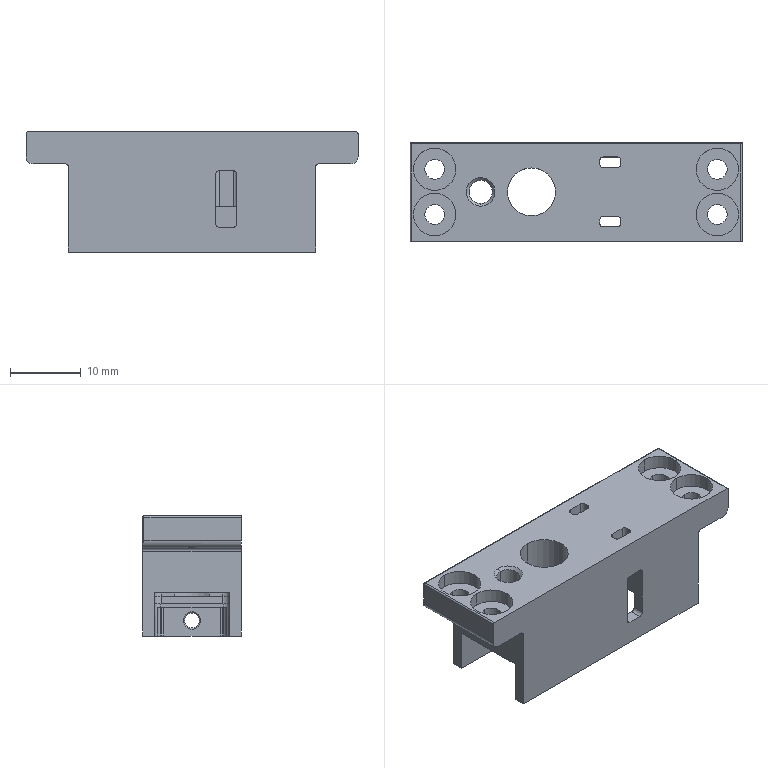NC program | NX | posted with a generic post | part box 47 x 14 x 17 mm
Lines 6223 to 7148 of 12912:
(CAVITY_MILL_COPY_COPY_COPY , TOOL : D1)
N12390 T22 M6
N12392 G54
N12394 G17 G0 G90 X9.057 Y-4.65 B0. C0. S9200 M3
N12396 G43 Z30. H22
N12398 Z0.936
N12400 G94 G1 Z-0.064 F1000.
N12402 G3 X9.492 Y-4.75 R1.
N12404 G1 X9.9 F850.
N12406 G3 X10.141 Y-4.628 R0.3
N12408 G2 X10.544 Y-4.425 R0.5
N12410 G1 X10.7
N12412 G3 X10.981 Y-4.231 R0.3
N12414 G2 X11.293 Y-3.885 R0.64
N12416 G3 X11.732 Y-3.456 R1.
N12418 G1 Z0.936
N12420 G0 Z30.
N12422 X9.057 Y-4.65
N12424 Z0.872
N12426 G1 Z-0.128 F1000.
N12428 G3 X9.492 Y-4.75 R1.
N12430 G1 X9.9 F850.
N12432 G3 X10.141 Y-4.628 R0.3
N12434 G2 X10.544 Y-4.425 R0.5
N12436 G1 X10.7
N12438 G3 X10.981 Y-4.231 R0.3
N12440 G2 X11.293 Y-3.885 R0.64
N12442 G3 X11.732 Y-3.456 R1.
N12444 G1 Z0.872
N12446 G0 Z30.
N12448 X9.057 Y-4.65
N12450 Z0.808
N12452 G1 Z-0.192 F1000.
N12454 G3 X9.492 Y-4.75 R1.
N12456 G1 X9.9 F850.
N12458 G3 X10.141 Y-4.628 R0.3
N12460 G2 X10.544 Y-4.425 R0.5
N12462 G1 X10.7
N12464 G3 X10.981 Y-4.231 R0.3
N12466 G2 X11.293 Y-3.885 R0.64
N12468 G3 X11.732 Y-3.456 R1.
N12470 G1 Z0.808
N12472 G0 Z30.
N12474 X9.057 Y-4.65
N12476 Z0.744
N12478 G1 Z-0.256 F1000.
N12480 G3 X9.492 Y-4.75 R1.
N12482 G1 X9.9 F850.
N12484 G3 X10.141 Y-4.628 R0.3
N12486 G2 X10.544 Y-4.425 R0.5
N12488 G1 X10.7
N12490 G3 X10.981 Y-4.231 R0.3
N12492 G2 X11.293 Y-3.885 R0.64
N12494 G3 X11.732 Y-3.456 R1.
N12496 G1 Z0.744
N12498 G0 Z30.
N12500 X9.057 Y-4.65
N12502 Z0.68
N12504 G1 Z-0.32 F1000.
N12506 G3 X9.492 Y-4.75 R1.
N12508 G1 X9.9 F850.
N12510 G3 X10.141 Y-4.628 R0.3
N12512 G2 X10.544 Y-4.425 R0.5
N12514 G1 X10.7
N12516 G3 X10.981 Y-4.231 R0.3
N12518 G2 X11.293 Y-3.885 R0.64
N12520 G3 X11.732 Y-3.456 R1.
N12522 G1 Z0.68
N12524 G0 Z30.
N12526 X9.057 Y-4.65
N12528 Z0.616
N12530 G1 Z-0.384 F1000.
N12532 G3 X9.492 Y-4.75 R1.
N12534 G1 X9.9 F850.
N12536 G3 X10.141 Y-4.628 R0.3
N12538 G2 X10.544 Y-4.425 R0.5
N12540 G1 X10.7
N12542 G3 X10.981 Y-4.231 R0.3
N12544 G2 X11.293 Y-3.885 R0.64
N12546 G3 X11.732 Y-3.456 R1.
N12548 G1 Z0.616
N12550 G0 Z30.
N12552 X9.057 Y-4.65
N12554 Z0.552
N12556 G1 Z-0.448 F1000.
N12558 G3 X9.492 Y-4.75 R1.
N12560 G1 X9.9 F850.
N12562 G3 X10.141 Y-4.628 R0.3
N12564 G2 X10.544 Y-4.425 R0.5
N12566 G1 X10.7
N12568 G3 X10.981 Y-4.231 R0.3
N12570 G2 X11.293 Y-3.885 R0.64
N12572 G3 X11.732 Y-3.456 R1.
N12574 G1 Z0.552
N12576 G0 Z30.
N12578 X9.057 Y-4.65
N12580 Z0.488
N12582 G1 Z-0.513 F1000.
N12584 G3 X9.492 Y-4.75 R1.
N12586 G1 X9.9 F850.
N12588 G3 X10.141 Y-4.628 R0.3
N12590 G2 X10.544 Y-4.425 R0.5
N12592 G1 X10.7
N12594 G3 X10.981 Y-4.231 R0.3
N12596 G2 X11.293 Y-3.885 R0.64
N12598 G3 X11.732 Y-3.456 R1.
N12600 G1 Z0.488
N12602 G0 Z30.
N12604 X9.057 Y-4.65
N12606 Z0.423
N12608 G1 Z-0.577 F1000.
N12610 G3 X9.492 Y-4.75 R1.
N12612 G1 X9.9 F850.
N12614 G3 X10.141 Y-4.628 R0.3
N12616 G2 X10.544 Y-4.425 R0.5
N12618 G1 X10.7
N12620 G3 X10.981 Y-4.231 R0.3
N12622 G2 X11.293 Y-3.885 R0.64
N12624 G3 X11.732 Y-3.456 R1.
N12626 G1 Z0.423
N12628 G0 Z30.
N12630 X9.057 Y-4.65
N12632 Z0.359
N12634 G1 Z-0.641 F1000.
N12636 G3 X9.492 Y-4.75 R1.
N12638 G1 X9.9 F850.
N12640 G3 X10.141 Y-4.628 R0.3
N12642 G2 X10.544 Y-4.425 R0.5
N12644 G1 X10.7
N12646 G3 X10.981 Y-4.231 R0.3
N12648 G2 X11.293 Y-3.885 R0.64
N12650 G3 X11.732 Y-3.456 R1.
N12652 G1 Z0.359
N12654 G0 Z30.
N12656 X9.057 Y-4.65
N12658 Z0.295
N12660 G1 Z-0.705 F1000.
N12662 G3 X9.492 Y-4.75 R1.
N12664 G1 X9.9 F850.
N12666 G3 X10.141 Y-4.628 R0.3
N12668 G2 X10.544 Y-4.425 R0.5
N12670 G1 X10.7
N12672 G3 X10.981 Y-4.231 R0.3
N12674 G2 X11.293 Y-3.885 R0.64
N12676 G3 X11.732 Y-3.456 R1.
N12678 G1 Z0.295
N12680 G0 Z30.
N12682 X9.057 Y-4.65
N12684 Z0.231
N12686 G1 Z-0.769 F1000.
N12688 G3 X9.492 Y-4.75 R1.
N12690 G1 X9.9 F850.
N12692 G3 X10.141 Y-4.628 R0.3
N12694 G2 X10.544 Y-4.425 R0.5
N12696 G1 X10.7
N12698 G3 X10.981 Y-4.231 R0.3
N12700 G2 X11.293 Y-3.885 R0.64
N12702 G3 X11.732 Y-3.456 R1.
N12704 G1 Z0.231
N12706 G0 Z30.
N12708 X9.057 Y-4.65
N12710 Z0.167
N12712 G1 Z-0.833 F1000.
N12714 G3 X9.492 Y-4.75 R1.
N12716 G1 X9.9 F850.
N12718 G3 X10.141 Y-4.628 R0.3
N12720 G2 X10.544 Y-4.425 R0.5
N12722 G1 X10.7
N12724 G3 X10.981 Y-4.231 R0.3
N12726 G2 X11.293 Y-3.885 R0.64
N12728 G3 X11.732 Y-3.456 R1.
N12730 G1 Z0.167
N12732 G0 Z30.
N12734 X9.057 Y-4.65
N12736 Z0.103
N12738 G1 Z-0.897 F1000.
N12740 G3 X9.492 Y-4.75 R1.
N12742 G1 X9.9 F850.
N12744 G3 X10.141 Y-4.628 R0.3
N12746 G2 X10.544 Y-4.425 R0.5
N12748 G1 X10.7
N12750 G3 X10.981 Y-4.231 R0.3
N12752 G2 X11.293 Y-3.885 R0.64
N12754 G3 X11.732 Y-3.456 R1.
N12756 G1 Z0.103
N12758 G0 Z30.
N12760 X9.057 Y-4.65
N12762 Z0.039
N12764 G1 Z-0.961 F1000.
N12766 G3 X9.492 Y-4.75 R1.
N12768 G1 X9.9 F850.
N12770 G3 X10.141 Y-4.628 R0.3
N12772 G2 X10.544 Y-4.425 R0.5
N12774 G1 X10.7
N12776 G3 X10.981 Y-4.231 R0.3
N12778 G2 X11.293 Y-3.885 R0.64
N12780 G3 X11.732 Y-3.456 R1.
N12782 G1 Z0.039
N12784 X9.057 Y-4.65 Z-0.025 F8000.
N12786 Z-1.025 F1000.
N12788 G3 X9.492 Y-4.75 R1.
N12790 G1 X9.9 F850.
N12792 G3 X10.141 Y-4.628 R0.3
N12794 G2 X10.544 Y-4.425 R0.5
N12796 G1 X10.7
N12798 G3 X10.981 Y-4.231 R0.3
N12800 G2 X11.293 Y-3.885 R0.64
N12802 G3 X11.732 Y-3.456 R1.
N12804 G1 Z-0.025
N12806 X9.057 Y-4.65 Z-0.089 F8000.
N12808 Z-1.089 F1000.
N12810 G3 X9.492 Y-4.75 R1.
N12812 G1 X9.9 F850.
N12814 G3 X10.141 Y-4.628 R0.3
N12816 G2 X10.544 Y-4.425 R0.5
N12818 G1 X10.7
N12820 G3 X10.981 Y-4.231 R0.3
N12822 G2 X11.293 Y-3.885 R0.64
N12824 G3 X11.732 Y-3.456 R1.
N12826 G1 Z-0.089
N12828 X9.057 Y-4.65 Z-0.153 F8000.
N12830 Z-1.153 F1000.
N12832 G3 X9.492 Y-4.75 R1.
N12834 G1 X9.9 F850.
N12836 G3 X10.141 Y-4.628 R0.3
N12838 G2 X10.544 Y-4.425 R0.5
N12840 G1 X10.7
N12842 G3 X10.981 Y-4.231 R0.3
N12844 G2 X11.293 Y-3.885 R0.64
N12846 G3 X11.732 Y-3.456 R1.
N12848 G1 Z-0.153
N12850 X9.057 Y-4.65 Z-0.217 F8000.
N12852 Z-1.217 F1000.
N12854 G3 X9.492 Y-4.75 R1.
N12856 G1 X9.9 F850.
N12858 G3 X10.141 Y-4.628 R0.3
N12860 G2 X10.544 Y-4.425 R0.5
N12862 G1 X10.7
N12864 G3 X10.981 Y-4.231 R0.3
N12866 G2 X11.293 Y-3.885 R0.64
N12868 G3 X11.732 Y-3.456 R1.
N12870 G1 Z-0.217
N12872 X9.057 Y-4.65 Z-0.281 F8000.
N12874 Z-1.281 F1000.
N12876 G3 X9.492 Y-4.75 R1.
N12878 G1 X9.9 F850.
N12880 G3 X10.141 Y-4.628 R0.3
N12882 G2 X10.544 Y-4.425 R0.5
N12884 G1 X10.7
N12886 G3 X10.981 Y-4.231 R0.3
N12888 G2 X11.293 Y-3.885 R0.64
N12890 G3 X11.732 Y-3.456 R1.
N12892 G1 Z-0.281
N12894 X9.057 Y-4.65 Z-0.345 F8000.
N12896 Z-1.345 F1000.
N12898 G3 X9.492 Y-4.75 R1.
N12900 G1 X9.9 F850.
N12902 G3 X10.141 Y-4.628 R0.3
N12904 G2 X10.544 Y-4.425 R0.5
N12906 G1 X10.7
N12908 G3 X10.981 Y-4.231 R0.3
N12910 G2 X11.293 Y-3.885 R0.64
N12912 G3 X11.732 Y-3.456 R1.
N12914 G1 Z-0.345
N12916 X9.057 Y-4.65 Z-0.409 F8000.
N12918 Z-1.409 F1000.
N12920 G3 X9.492 Y-4.75 R1.
N12922 G1 X9.9 F850.
N12924 G3 X10.141 Y-4.628 R0.3
N12926 G2 X10.544 Y-4.425 R0.5
N12928 G1 X10.71
N12930 G3 X10.981 Y-4.231 R0.3
N12932 G2 X11.293 Y-3.885 R0.64
N12934 G3 X11.732 Y-3.456 R1.
N12936 G1 Z-0.409
N12938 X9.057 Y-4.65 Z-0.473 F8000.
N12940 Z-1.473 F1000.
N12942 G3 X9.492 Y-4.75 R1.
N12944 G1 X9.9 F850.
N12946 G3 X10.141 Y-4.628 R0.3
N12948 G2 X10.544 Y-4.425 R0.5
N12950 G1 X10.71
N12952 G3 X10.981 Y-4.231 R0.3
N12954 G2 X11.293 Y-3.885 R0.64
N12956 G3 X11.732 Y-3.456 R1.
N12958 G1 Z-0.473
N12960 X9.057 Y-4.65 Z-0.538 F8000.
N12962 Z-1.538 F1000.
N12964 G3 X9.492 Y-4.75 R1.
N12966 G1 X9.9 F850.
N12968 G3 X10.141 Y-4.628 R0.3
N12970 G2 X10.544 Y-4.425 R0.5
N12972 G1 X10.711
N12974 G3 X10.981 Y-4.231 R0.3
N12976 G2 X11.293 Y-3.885 R0.64
N12978 G3 X11.732 Y-3.456 R1.
N12980 G1 Z-0.538
N12982 X9.057 Y-4.65 Z-0.602 F8000.
N12984 Z-1.602 F1000.
N12986 G3 X9.492 Y-4.75 R1.
N12988 G1 X9.9 F850.
N12990 G3 X10.141 Y-4.628 R0.3
N12992 G2 X10.544 Y-4.425 R0.5
N12994 G1 X10.711
N12996 G3 X10.981 Y-4.231 R0.3
N12998 G2 X11.293 Y-3.885 R0.64
N13000 G3 X11.732 Y-3.456 R1.
N13002 G1 Z-0.602
N13004 X9.057 Y-4.65 Z-0.666 F8000.
N13006 Z-1.666 F1000.
N13008 G3 X9.492 Y-4.75 R1.
N13010 G1 X9.9 F850.
N13012 G3 X10.141 Y-4.628 R0.3
N13014 G2 X10.544 Y-4.425 R0.5
N13016 G1 X10.711
N13018 G3 X10.981 Y-4.231 R0.3
N13020 G2 X11.293 Y-3.885 R0.64
N13022 G3 X11.732 Y-3.456 R1.
N13024 G1 Z-0.666
N13026 X9.057 Y-4.65 Z-0.73 F8000.
N13028 Z-1.73 F1000.
N13030 G3 X9.492 Y-4.75 R1.
N13032 G1 X9.9 F850.
N13034 G3 X10.141 Y-4.628 R0.3
N13036 G2 X10.544 Y-4.425 R0.5
N13038 G1 X10.711
N13040 G3 X10.981 Y-4.231 R0.3
N13042 G2 X11.293 Y-3.885 R0.64
N13044 G3 X11.732 Y-3.456 R1.
N13046 G1 Z-0.73
N13048 X9.057 Y-4.65 Z-0.794 F8000.
N13050 Z-1.794 F1000.
N13052 G3 X9.492 Y-4.75 R1.
N13054 G1 X9.9 F850.
N13056 G3 X10.141 Y-4.628 R0.3
N13058 G2 X10.544 Y-4.425 R0.5
N13060 G1 X10.711
N13062 G3 X10.981 Y-4.231 R0.3
N13064 G2 X11.293 Y-3.885 R0.64
N13066 G3 X11.732 Y-3.456 R1.
N13068 G1 Z-0.794
N13070 X9.057 Y-4.65 Z-0.858 F8000.
N13072 Z-1.858 F1000.
N13074 G3 X9.492 Y-4.75 R1.
N13076 G1 X9.9 F850.
N13078 G3 X10.141 Y-4.628 R0.3
N13080 G2 X10.544 Y-4.425 R0.5
N13082 G1 X10.712
N13084 G3 X10.981 Y-4.231 R0.3
N13086 G2 X11.293 Y-3.885 R0.64
N13088 G3 X11.732 Y-3.456 R1.
N13090 G1 Z-0.858
N13092 X9.057 Y-4.65 Z-0.922 F8000.
N13094 Z-1.922 F1000.
N13096 G3 X9.492 Y-4.75 R1.
N13098 G1 X9.9 F850.
N13100 G3 X10.141 Y-4.628 R0.3
N13102 G2 X10.544 Y-4.425 R0.5
N13104 G1 X10.712
N13106 G3 X10.981 Y-4.231 R0.3
N13108 G2 X11.293 Y-3.885 R0.64
N13110 G3 X11.732 Y-3.456 R1.
N13112 G1 Z-0.922
N13114 X9.057 Y-4.65 Z-0.986 F8000.
N13116 Z-1.986 F1000.
N13118 G3 X9.492 Y-4.75 R1.
N13120 G1 X9.9 F850.
N13122 G3 X10.141 Y-4.628 R0.3
N13124 G2 X10.544 Y-4.425 R0.5
N13126 G1 X10.712
N13128 G3 X10.981 Y-4.231 R0.3
N13130 G2 X11.293 Y-3.885 R0.64
N13132 G3 X11.732 Y-3.456 R1.
N13134 G1 Z-0.986
N13136 X9.057 Y-4.65 Z-1.05 F8000.
N13138 Z-2.05 F1000.
N13140 G3 X9.492 Y-4.75 R1.
N13142 G1 X9.9 F850.
N13144 G3 X10.141 Y-4.628 R0.3
N13146 G2 X10.544 Y-4.425 R0.5
N13148 G1 X10.712
N13150 G3 X10.981 Y-4.231 R0.3
N13152 G2 X11.293 Y-3.885 R0.64
N13154 G3 X11.732 Y-3.456 R1.
N13156 G1 Z-1.05
N13158 X9.057 Y-4.65 Z-1.114 F8000.
N13160 Z-2.114 F1000.
N13162 G3 X9.492 Y-4.75 R1.
N13164 G1 X9.9 F850.
N13166 G3 X10.141 Y-4.628 R0.3
N13168 G2 X10.544 Y-4.425 R0.5
N13170 G1 X10.712
N13172 G3 X10.981 Y-4.231 R0.3
N13174 G2 X11.293 Y-3.885 R0.64
N13176 G3 X11.732 Y-3.456 R1.
N13178 G1 Z-1.114
N13180 X9.057 Y-4.65 Z-1.178 F8000.
N13182 Z-2.178 F1000.
N13184 G3 X9.492 Y-4.75 R1.
N13186 G1 X9.9 F850.
N13188 G3 X10.141 Y-4.628 R0.3
N13190 G2 X10.544 Y-4.425 R0.5
N13192 G1 X10.713
N13194 G3 X10.981 Y-4.231 R0.3
N13196 G2 X11.293 Y-3.885 R0.64
N13198 G3 X11.732 Y-3.456 R1.
N13200 G1 Z-1.178
N13202 X9.057 Y-4.65 Z-1.242 F8000.
N13204 Z-2.242 F1000.
N13206 G3 X9.492 Y-4.75 R1.
N13208 G1 X9.9 F850.
N13210 G3 X10.141 Y-4.628 R0.3
N13212 G2 X10.544 Y-4.425 R0.5
N13214 G1 X10.713
N13216 G3 X10.981 Y-4.231 R0.3
N13218 G2 X11.293 Y-3.885 R0.64
N13220 G3 X11.732 Y-3.456 R1.
N13222 G1 Z-1.242
N13224 X9.057 Y-4.65 Z-1.306 F8000.
N13226 Z-2.306 F1000.
N13228 G3 X9.492 Y-4.75 R1.
N13230 G1 X9.9 F850.
N13232 G3 X10.141 Y-4.628 R0.3
N13234 G2 X10.544 Y-4.425 R0.5
N13236 G1 X10.713
N13238 G3 X10.981 Y-4.231 R0.3
N13240 G2 X11.293 Y-3.885 R0.64
N13242 G3 X11.732 Y-3.456 R1.
N13244 G1 Z-1.306
N13246 X9.057 Y-4.65 Z-1.37 F8000.
N13248 Z-2.37 F1000.
N13250 G3 X9.492 Y-4.75 R1.
N13252 G1 X9.9 F850.
N13254 G3 X10.141 Y-4.628 R0.3
N13256 G2 X10.544 Y-4.425 R0.5
N13258 G1 X10.713
N13260 G3 X10.981 Y-4.231 R0.3
N13262 G2 X11.293 Y-3.885 R0.64
N13264 G3 X11.732 Y-3.456 R1.
N13266 G1 Z-1.37
N13268 X9.057 Y-4.65 Z-1.434 F8000.
N13270 Z-2.434 F1000.
N13272 G3 X9.492 Y-4.75 R1.
N13274 G1 X9.9 F850.
N13276 G3 X10.141 Y-4.628 R0.3
N13278 G2 X10.544 Y-4.425 R0.5
N13280 G1 X10.713
N13282 G3 X10.981 Y-4.231 R0.3
N13284 G2 X11.293 Y-3.885 R0.64
N13286 G3 X11.732 Y-3.456 R1.
N13288 G1 Z-1.434
N13290 X9.057 Y-4.65 Z-1.498 F8000.
N13292 Z-2.498 F1000.
N13294 G3 X9.492 Y-4.75 R1.
N13296 G1 X9.9 F850.
N13298 G3 X10.141 Y-4.628 R0.3
N13300 G2 X10.544 Y-4.425 R0.5
N13302 G1 X10.714
N13304 G3 X10.981 Y-4.231 R0.3
N13306 G2 X11.293 Y-3.885 R0.64
N13308 G3 X11.732 Y-3.456 R1.
N13310 G1 Z-1.498
N13312 X9.057 Y-4.65 Z-1.563 F8000.
N13314 Z-2.563 F1000.
N13316 G3 X9.492 Y-4.75 R1.
N13318 G1 X9.9 F850.
N13320 G3 X10.141 Y-4.628 R0.3
N13322 G2 X10.544 Y-4.425 R0.5
N13324 G1 X10.714
N13326 G3 X10.981 Y-4.231 R0.3
N13328 G2 X11.293 Y-3.885 R0.64
N13330 G3 X11.732 Y-3.456 R1.
N13332 G1 Z-1.563
N13334 X9.057 Y-4.65 Z-1.627 F8000.
N13336 Z-2.627 F1000.
N13338 G3 X9.492 Y-4.75 R1.
N13340 G1 X9.9 F850.
N13342 G3 X10.141 Y-4.628 R0.3
N13344 G2 X10.544 Y-4.425 R0.5
N13346 G1 X10.714
N13348 G3 X10.981 Y-4.231 R0.3
N13350 G2 X11.293 Y-3.885 R0.64
N13352 G3 X11.732 Y-3.456 R1.
N13354 G1 Z-1.627
N13356 X9.057 Y-4.65 Z-1.691 F8000.
N13358 Z-2.691 F1000.
N13360 G3 X9.492 Y-4.75 R1.
N13362 G1 X9.9 F850.
N13364 G3 X10.141 Y-4.628 R0.3
N13366 G2 X10.544 Y-4.425 R0.5
N13368 G1 X10.714
N13370 G3 X10.981 Y-4.231 R0.3
N13372 G2 X11.293 Y-3.885 R0.64
N13374 G3 X11.732 Y-3.456 R1.
N13376 G1 Z-1.691
N13378 X9.057 Y-4.65 Z-1.755 F8000.
N13380 Z-2.755 F1000.
N13382 G3 X9.492 Y-4.75 R1.
N13384 G1 X9.9 F850.
N13386 G3 X10.141 Y-4.628 R0.3
N13388 G2 X10.544 Y-4.425 R0.5
N13390 G1 X10.714
N13392 G3 X10.981 Y-4.231 R0.3
N13394 G2 X11.293 Y-3.885 R0.64
N13396 G3 X11.732 Y-3.456 R1.
N13398 G1 Z-1.755
N13400 X9.057 Y-4.65 Z-1.819 F8000.
N13402 Z-2.819 F1000.
N13404 G3 X9.492 Y-4.75 R1.
N13406 G1 X9.9 F850.
N13408 G3 X10.141 Y-4.628 R0.3
N13410 G2 X10.544 Y-4.425 R0.5
N13412 G1 X10.714
N13414 G3 X10.981 Y-4.231 R0.3
N13416 G2 X11.293 Y-3.885 R0.64
N13418 G3 X11.732 Y-3.456 R1.
N13420 G1 Z-1.819
N13422 X9.057 Y-4.65 Z-1.883 F8000.
N13424 Z-2.883 F1000.
N13426 G3 X9.492 Y-4.75 R1.
N13428 G1 X9.9 F850.
N13430 G3 X10.141 Y-4.628 R0.3
N13432 G2 X10.544 Y-4.425 R0.5
N13434 G1 X10.715
N13436 G3 X10.981 Y-4.231 R0.3
N13438 G2 X11.293 Y-3.885 R0.64
N13440 G3 X11.732 Y-3.456 R1.
N13442 G1 Z-1.883
N13444 X9.057 Y-4.65 Z-1.947 F8000.
N13446 Z-2.947 F1000.
N13448 G3 X9.492 Y-4.75 R1.
N13450 G1 X9.9 F850.
N13452 G3 X10.141 Y-4.628 R0.3
N13454 G2 X10.544 Y-4.425 R0.5
N13456 G1 X10.715
N13458 G3 X10.981 Y-4.231 R0.3
N13460 G2 X11.293 Y-3.885 R0.64
N13462 G3 X11.732 Y-3.456 R1.
N13464 G1 Z-1.947
N13466 X9.057 Y-4.65 Z-2.011 F8000.
N13468 Z-3.011 F1000.
N13470 G3 X9.492 Y-4.75 R1.
N13472 G1 X9.9 F850.
N13474 G3 X10.141 Y-4.628 R0.3
N13476 G2 X10.544 Y-4.425 R0.5
N13478 G1 X10.715
N13480 G3 X10.981 Y-4.231 R0.3
N13482 G2 X11.293 Y-3.885 R0.64
N13484 G3 X11.732 Y-3.456 R1.
N13486 G1 Z-2.011
N13488 X9.057 Y-4.65 Z-2.075 F8000.
N13490 Z-3.075 F1000.
N13492 G3 X9.492 Y-4.75 R1.
N13494 G1 X9.9 F850.
N13496 G3 X10.141 Y-4.628 R0.3
N13498 G2 X10.544 Y-4.425 R0.5
N13500 G1 X10.715
N13502 G3 X10.981 Y-4.231 R0.3
N13504 G2 X11.293 Y-3.885 R0.64
N13506 G3 X11.732 Y-3.456 R1.
N13508 G1 Z-2.075
N13510 X9.057 Y-4.65 Z-2.139 F8000.
N13512 Z-3.139 F1000.
N13514 G3 X9.492 Y-4.75 R1.
N13516 G1 X9.9 F850.
N13518 G3 X10.141 Y-4.628 R0.3
N13520 G2 X10.544 Y-4.425 R0.5
N13522 G1 X10.715
N13524 G3 X10.981 Y-4.231 R0.3
N13526 G2 X11.293 Y-3.885 R0.64
N13528 G3 X11.732 Y-3.456 R1.
N13530 G1 Z-2.139
N13532 X9.057 Y-4.65 Z-2.203 F8000.
N13534 Z-3.203 F1000.
N13536 G3 X9.492 Y-4.75 R1.
N13538 G1 X9.9 F850.
N13540 G3 X10.141 Y-4.628 R0.3
N13542 G2 X10.544 Y-4.425 R0.5
N13544 G1 X10.715
N13546 G3 X10.981 Y-4.231 R0.3
N13548 G2 X11.293 Y-3.885 R0.64
N13550 G3 X11.732 Y-3.456 R1.
N13552 G1 Z-2.203
N13554 X9.057 Y-4.65 Z-2.267 F8000.
N13556 Z-3.267 F1000.
N13558 G3 X9.492 Y-4.75 R1.
N13560 G1 X9.9 F850.
N13562 G3 X10.141 Y-4.628 R0.3
N13564 G2 X10.544 Y-4.425 R0.5
N13566 G1 X10.715
N13568 G3 X10.981 Y-4.231 R0.3
N13570 G2 X11.293 Y-3.885 R0.64
N13572 G3 X11.732 Y-3.456 R1.
N13574 G1 Z-2.267
N13576 X9.057 Y-4.65 Z-2.331 F8000.
N13578 Z-3.331 F1000.
N13580 G3 X9.492 Y-4.75 R1.
N13582 G1 X9.9 F850.
N13584 G3 X10.141 Y-4.628 R0.3
N13586 G2 X10.544 Y-4.425 R0.5
N13588 G1 X10.716
N13590 G3 X10.981 Y-4.231 R0.3
N13592 G2 X11.293 Y-3.885 R0.64
N13594 G3 X11.732 Y-3.456 R1.
N13596 G1 Z-2.331
N13598 X9.057 Y-4.65 Z-2.395 F8000.
N13600 Z-3.395 F1000.
N13602 G3 X9.492 Y-4.75 R1.
N13604 G1 X9.9 F850.
N13606 G3 X10.141 Y-4.628 R0.3
N13608 G2 X10.544 Y-4.425 R0.5
N13610 G1 X10.716
N13612 G3 X10.981 Y-4.231 R0.3
N13614 G2 X11.293 Y-3.885 R0.64
N13616 G3 X11.732 Y-3.456 R1.
N13618 G1 Z-2.395
N13620 X9.057 Y-4.65 Z-2.459 F8000.
N13622 Z-3.459 F1000.
N13624 G3 X9.492 Y-4.75 R1.
N13626 G1 X9.9 F850.
N13628 G3 X10.141 Y-4.628 R0.3
N13630 G2 X10.544 Y-4.425 R0.5
N13632 G1 X10.716
N13634 G3 X10.981 Y-4.231 R0.3
N13636 G2 X11.293 Y-3.885 R0.64
N13638 G3 X11.732 Y-3.456 R1.
N13640 G1 Z-2.459
N13642 X9.057 Y-4.65 Z-2.523 F8000.
N13644 Z-3.523 F1000.
N13646 G3 X9.492 Y-4.75 R1.
N13648 G1 X9.9 F850.
N13650 G3 X10.141 Y-4.628 R0.3
N13652 G2 X10.544 Y-4.425 R0.5
N13654 G1 X10.716
N13656 G3 X10.981 Y-4.231 R0.3
N13658 G2 X11.293 Y-3.885 R0.64
N13660 G3 X11.732 Y-3.456 R1.
N13662 G1 Z-2.523
N13664 X9.057 Y-4.65 Z-2.588 F8000.
N13666 Z-3.588 F1000.
N13668 G3 X9.492 Y-4.75 R1.
N13670 G1 X9.9 F850.
N13672 G3 X10.141 Y-4.628 R0.3
N13674 G2 X10.544 Y-4.425 R0.5
N13676 G1 X10.716
N13678 G3 X10.981 Y-4.231 R0.3
N13680 G2 X11.293 Y-3.885 R0.64
N13682 G3 X11.732 Y-3.456 R1.
N13684 G1 Z-2.588
N13686 X9.057 Y-4.65 Z-2.652 F8000.
N13688 Z-3.652 F1000.
N13690 G3 X9.492 Y-4.75 R1.
N13692 G1 X9.9 F850.
N13694 G3 X10.141 Y-4.628 R0.3
N13696 G2 X10.544 Y-4.425 R0.5
N13698 G1 X10.716
N13700 G3 X10.981 Y-4.231 R0.3
N13702 G2 X11.293 Y-3.885 R0.64
N13704 G3 X11.732 Y-3.456 R1.
N13706 G1 Z-2.652
N13708 X9.057 Y-4.65 Z-2.716 F8000.
N13710 Z-3.716 F1000.
N13712 G3 X9.492 Y-4.75 R1.
N13714 G1 X9.9 F850.
N13716 G3 X10.141 Y-4.628 R0.3
N13718 G2 X10.544 Y-4.425 R0.5
N13720 G1 X10.716
N13722 G3 X10.981 Y-4.231 R0.3
N13724 G2 X11.293 Y-3.885 R0.64
N13726 G3 X11.732 Y-3.456 R1.
N13728 G1 Z-2.716
N13730 X9.057 Y-4.65 Z-2.78 F8000.
N13732 Z-3.78 F1000.
N13734 G3 X9.492 Y-4.75 R1.
N13736 G1 X9.9 F850.
N13738 G3 X10.141 Y-4.628 R0.3
N13740 G2 X10.544 Y-4.425 R0.5
N13742 G1 X10.717
N13744 G3 X10.981 Y-4.231 R0.3
N13746 G2 X11.293 Y-3.885 R0.64
N13748 G3 X11.732 Y-3.456 R1.
N13750 G1 Z-2.78
N13752 X9.057 Y-4.65 Z-2.844 F8000.
N13754 Z-3.844 F1000.
N13756 G3 X9.492 Y-4.75 R1.
N13758 G1 X9.9 F850.
N13760 G3 X10.141 Y-4.628 R0.3
N13762 G2 X10.544 Y-4.425 R0.5
N13764 G1 X10.717
N13766 G3 X10.981 Y-4.231 R0.3
N13768 G2 X11.293 Y-3.885 R0.64
N13770 G3 X11.732 Y-3.456 R1.
N13772 G1 Z-2.844
N13774 X9.057 Y-4.65 Z-2.908 F8000.
N13776 Z-3.908 F1000.
N13778 G3 X9.492 Y-4.75 R1.
N13780 G1 X9.9 F850.
N13782 G3 X10.141 Y-4.628 R0.3
N13784 G2 X10.544 Y-4.425 R0.5
N13786 G1 X10.717
N13788 G3 X10.981 Y-4.231 R0.3
N13790 G2 X11.293 Y-3.885 R0.64
N13792 G3 X11.732 Y-3.456 R1.
N13794 G1 Z-2.908
N13796 X9.057 Y-4.65 Z-2.972 F8000.
N13798 Z-3.972 F1000.
N13800 G3 X9.492 Y-4.75 R1.
N13802 G1 X9.9 F850.
N13804 G3 X10.141 Y-4.628 R0.3
N13806 G2 X10.544 Y-4.425 R0.5
N13808 G1 X10.717
N13810 G3 X10.981 Y-4.231 R0.3
N13812 G2 X11.293 Y-3.885 R0.64
N13814 G3 X11.732 Y-3.456 R1.
N13816 G1 Z-2.972
N13818 X9.057 Y-4.65 Z-3.036 F8000.
N13820 Z-4.036 F1000.
N13822 G3 X9.492 Y-4.75 R1.
N13824 G1 X9.9 F850.
N13826 G3 X10.141 Y-4.628 R0.3
N13828 G2 X10.544 Y-4.425 R0.5
N13830 G1 X10.717
N13832 G3 X10.981 Y-4.231 R0.3
N13834 G2 X11.293 Y-3.885 R0.64
N13836 G3 X11.732 Y-3.456 R1.
N13838 G1 Z-3.036
N13840 X9.057 Y-4.65 Z-3.1 F8000.
N13842 Z-4.1 F1000.
N13844 G3 X9.492 Y-4.75 R1.
N13846 G1 X9.9 F850.
N13848 G3 X10.141 Y-4.628 R0.3
N13850 G2 X10.544 Y-4.425 R0.5
N13852 G1 X10.717
N13854 G3 X10.981 Y-4.231 R0.3
N13856 G2 X11.293 Y-3.885 R0.64
N13858 G3 X11.732 Y-3.456 R1.
N13860 G1 Z-3.1
N13862 X8.907 Y-4.65 Z-3.163 F8000.
N13864 Z-4.163 F1000.
N13866 G3 X9.343 Y-4.75 R1.
N13868 G1 X9.9 F850.
N13870 G3 X10.2 Y-4.45 R0.3
N13872 G1 Y-3.893
N13874 G3 X10.1 Y-3.457 R1.
N13876 G1 Z-3.163
N13878 X8.907 Y-4.65 Z-3.225 F8000.
N13880 Z-4.225 F1000.
N13882 G3 X9.343 Y-4.75 R1.
N13884 G1 X9.9 F850.
N13886 G3 X10.2 Y-4.45 R0.3
N13888 G1 Y-3.893
N13890 G3 X10.1 Y-3.457 R1.
N13892 G1 Z-3.225
N13894 X8.907 Y-4.65 Z-3.288 F8000.
N13896 Z-4.288 F1000.
N13898 G3 X9.343 Y-4.75 R1.
N13900 G1 X9.9 F850.
N13902 G3 X10.2 Y-4.45 R0.3
N13904 G1 Y-3.893
N13906 G3 X10.1 Y-3.457 R1.
N13908 G1 Z-3.288
N13910 X8.907 Y-4.65 Z-3.35 F8000.
N13912 Z-4.35 F1000.
N13914 G3 X9.343 Y-4.75 R1.
N13916 G1 X9.9 F850.
N13918 G3 X10.2 Y-4.45 R0.3
N13920 G1 Y-3.893
N13922 G3 X10.1 Y-3.457 R1.
N13924 G1 Z-3.35
N13926 X8.907 Y-4.65 Z-3.413 F8000.
N13928 Z-4.413 F1000.
N13930 G3 X9.343 Y-4.75 R1.
N13932 G1 X9.9 F850.
N13934 G3 X10.2 Y-4.45 R0.3
N13936 G1 Y-3.893
N13938 G3 X10.1 Y-3.457 R1.
N13940 G1 Z-3.413
N13942 X8.907 Y-4.65 Z-3.475 F8000.
N13944 Z-4.475 F1000.
N13946 G3 X9.343 Y-4.75 R1.
N13948 G1 X9.9 F850.
N13950 G3 X10.2 Y-4.45 R0.3
N13952 G1 Y-3.893
N13954 G3 X10.1 Y-3.457 R1.
N13956 G1 Z-3.475
N13958 X8.907 Y-4.65 Z-3.538 F8000.
N13960 Z-4.538 F1000.
N13962 G3 X9.343 Y-4.75 R1.
N13964 G1 X9.9 F850.
N13966 G3 X10.2 Y-4.45 R0.3
N13968 G1 Y-3.893
N13970 G3 X10.1 Y-3.457 R1.
N13972 G1 Z-3.538
N13974 X8.907 Y-4.65 Z-3.6 F8000.
N13976 Z-4.6 F1000.
N13978 G3 X9.343 Y-4.75 R1.
N13980 G1 X9.9 F850.
N13982 G3 X10.2 Y-4.45 R0.3
N13984 G1 Y-3.893
N13986 G3 X10.1 Y-3.457 R1.
N13988 G1 Z-3.6
N13990 X8.907 Y-4.65 Z-3.663 F8000.
N13992 Z-4.663 F1000.
N13994 G3 X9.343 Y-4.75 R1.
N13996 G1 X9.9 F850.
N13998 G3 X10.2 Y-4.45 R0.3
N14000 G1 Y-3.893
N14002 G3 X10.1 Y-3.457 R1.
N14004 G1 Z-3.663
N14006 X8.907 Y-4.65 Z-3.725 F8000.
N14008 Z-4.725 F1000.
N14010 G3 X9.343 Y-4.75 R1.
N14012 G1 X9.9 F850.
N14014 G3 X10.2 Y-4.45 R0.3
N14016 G1 Y-3.893
N14018 G3 X10.1 Y-3.457 R1.
N14020 G1 Z-3.725
N14022 X8.907 Y-4.65 Z-3.788 F8000.
N14024 Z-4.788 F1000.
N14026 G3 X9.343 Y-4.75 R1.
N14028 G1 X9.9 F850.
N14030 G3 X10.2 Y-4.45 R0.3
N14032 G1 Y-3.893
N14034 G3 X10.1 Y-3.457 R1.
N14036 G1 Z-3.788
N14038 X8.907 Y-4.65 Z-3.85 F8000.
N14040 Z-4.85 F1000.
N14042 G3 X9.343 Y-4.75 R1.
N14044 G1 X9.9 F850.
N14046 G3 X10.2 Y-4.45 R0.3
N14048 G1 Y-3.893
N14050 G3 X10.1 Y-3.457 R1.
N14052 G1 Z-3.85
N14054 X8.907 Y-4.65 Z-3.913 F8000.
N14056 Z-4.913 F1000.
N14058 G3 X9.343 Y-4.75 R1.
N14060 G1 X9.9 F850.
N14062 G3 X10.2 Y-4.45 R0.3
N14064 G1 Y-3.893
N14066 G3 X10.1 Y-3.457 R1.
N14068 G1 Z-3.913
N14070 X8.907 Y-4.65 Z-3.975 F8000.
N14072 Z-4.975 F1000.
N14074 G3 X9.343 Y-4.75 R1.
N14076 G1 X9.9 F850.
N14078 G3 X10.2 Y-4.45 R0.3
N14080 G1 Y-3.893
N14082 G3 X10.1 Y-3.457 R1.
N14084 G1 Z-3.975
N14086 X8.907 Y-4.65 Z-4.038 F8000.
N14088 Z-5.038 F1000.
N14090 G3 X9.343 Y-4.75 R1.
N14092 G1 X9.9 F850.
N14094 G3 X10.2 Y-4.45 R0.3
N14096 G1 Y-3.893
N14098 G3 X10.1 Y-3.457 R1.
N14100 G1 Z-4.038
N14102 X8.907 Y-4.65 Z-4.1 F8000.
N14104 Z-5.1 F1000.
N14106 G3 X9.343 Y-4.75 R1.
N14108 G1 X9.9 F850.
N14110 G3 X10.2 Y-4.45 R0.3
N14112 G1 Y-3.893
N14114 G3 X10.1 Y-3.457 R1.
N14116 G1 Z-4.1
N14118 X8.907 Y-4.65 Z-4.163 F8000.
N14120 Z-5.163 F1000.
N14122 G3 X9.343 Y-4.75 R1.
N14124 G1 X9.9 F850.
N14126 G3 X10.2 Y-4.45 R0.3
N14128 G1 Y-3.893
N14130 G3 X10.1 Y-3.457 R1.
N14132 G1 Z-4.163
N14134 X8.907 Y-4.65 Z-4.225 F8000.
N14136 Z-5.225 F1000.
N14138 G3 X9.343 Y-4.75 R1.
N14140 G1 X9.9 F850.
N14142 G3 X10.2 Y-4.45 R0.3
N14144 G1 Y-3.893
N14146 G3 X10.1 Y-3.457 R1.
N14148 G1 Z-4.225
N14150 X8.907 Y-4.65 Z-4.288 F8000.
N14152 Z-5.288 F1000.
N14154 G3 X9.343 Y-4.75 R1.
N14156 G1 X9.9 F850.
N14158 G3 X10.2 Y-4.45 R0.3
N14160 G1 Y-3.893
N14162 G3 X10.1 Y-3.457 R1.
N14164 G1 Z-4.288
N14166 X8.907 Y-4.65 Z-4.35 F8000.
N14168 Z-5.35 F1000.
N14170 G3 X9.343 Y-4.75 R1.
N14172 G1 X9.9 F850.
N14174 G3 X10.2 Y-4.45 R0.3
N14176 G1 Y-3.893
N14178 G3 X10.1 Y-3.457 R1.
N14180 G1 Z-4.35
N14182 X8.907 Y-4.65 Z-4.413 F8000.
N14184 Z-5.413 F1000.
N14186 G3 X9.343 Y-4.75 R1.
N14188 G1 X9.9 F850.
N14190 G3 X10.2 Y-4.45 R0.3
N14192 G1 Y-3.893
N14194 G3 X10.1 Y-3.457 R1.
N14196 G1 Z-4.413
N14198 X8.907 Y-4.65 Z-4.475 F8000.
N14200 Z-5.475 F1000.
N14202 G3 X9.343 Y-4.75 R1.
N14204 G1 X9.9 F850.
N14206 G3 X10.2 Y-4.45 R0.3
N14208 G1 Y-3.893
N14210 G3 X10.1 Y-3.457 R1.
N14212 G1 Z-4.475
N14214 X8.907 Y-4.65 Z-4.538 F8000.
N14216 Z-5.538 F1000.
N14218 G3 X9.343 Y-4.75 R1.
N14220 G1 X9.9 F850.
N14222 G3 X10.2 Y-4.45 R0.3
N14224 G1 Y-3.893
N14226 G3 X10.1 Y-3.457 R1.
N14228 G1 Z-4.538
N14230 X8.907 Y-4.65 Z-4.6 F8000.
N14232 Z-5.6 F1000.
N14234 G3 X9.343 Y-4.75 R1.